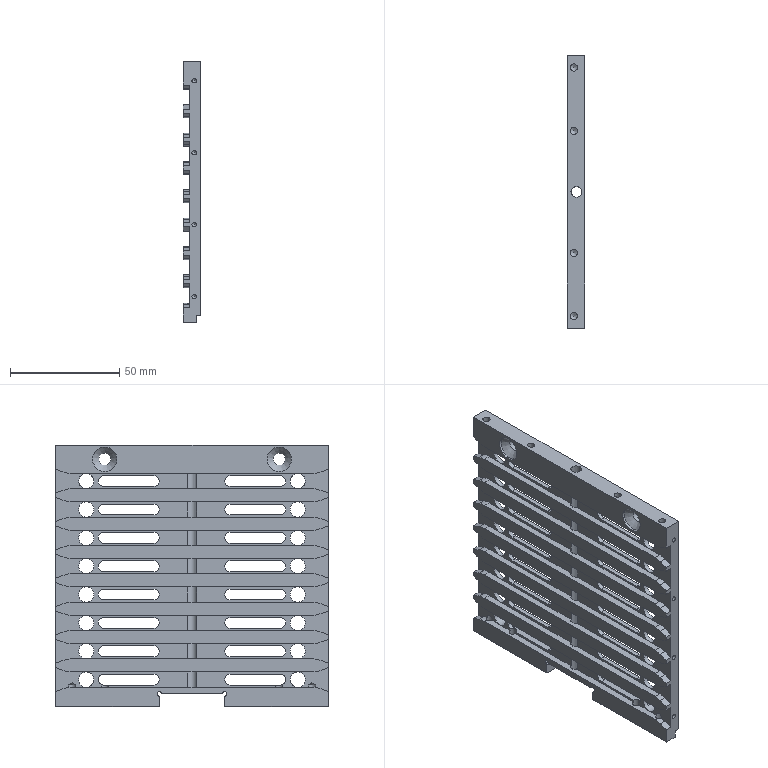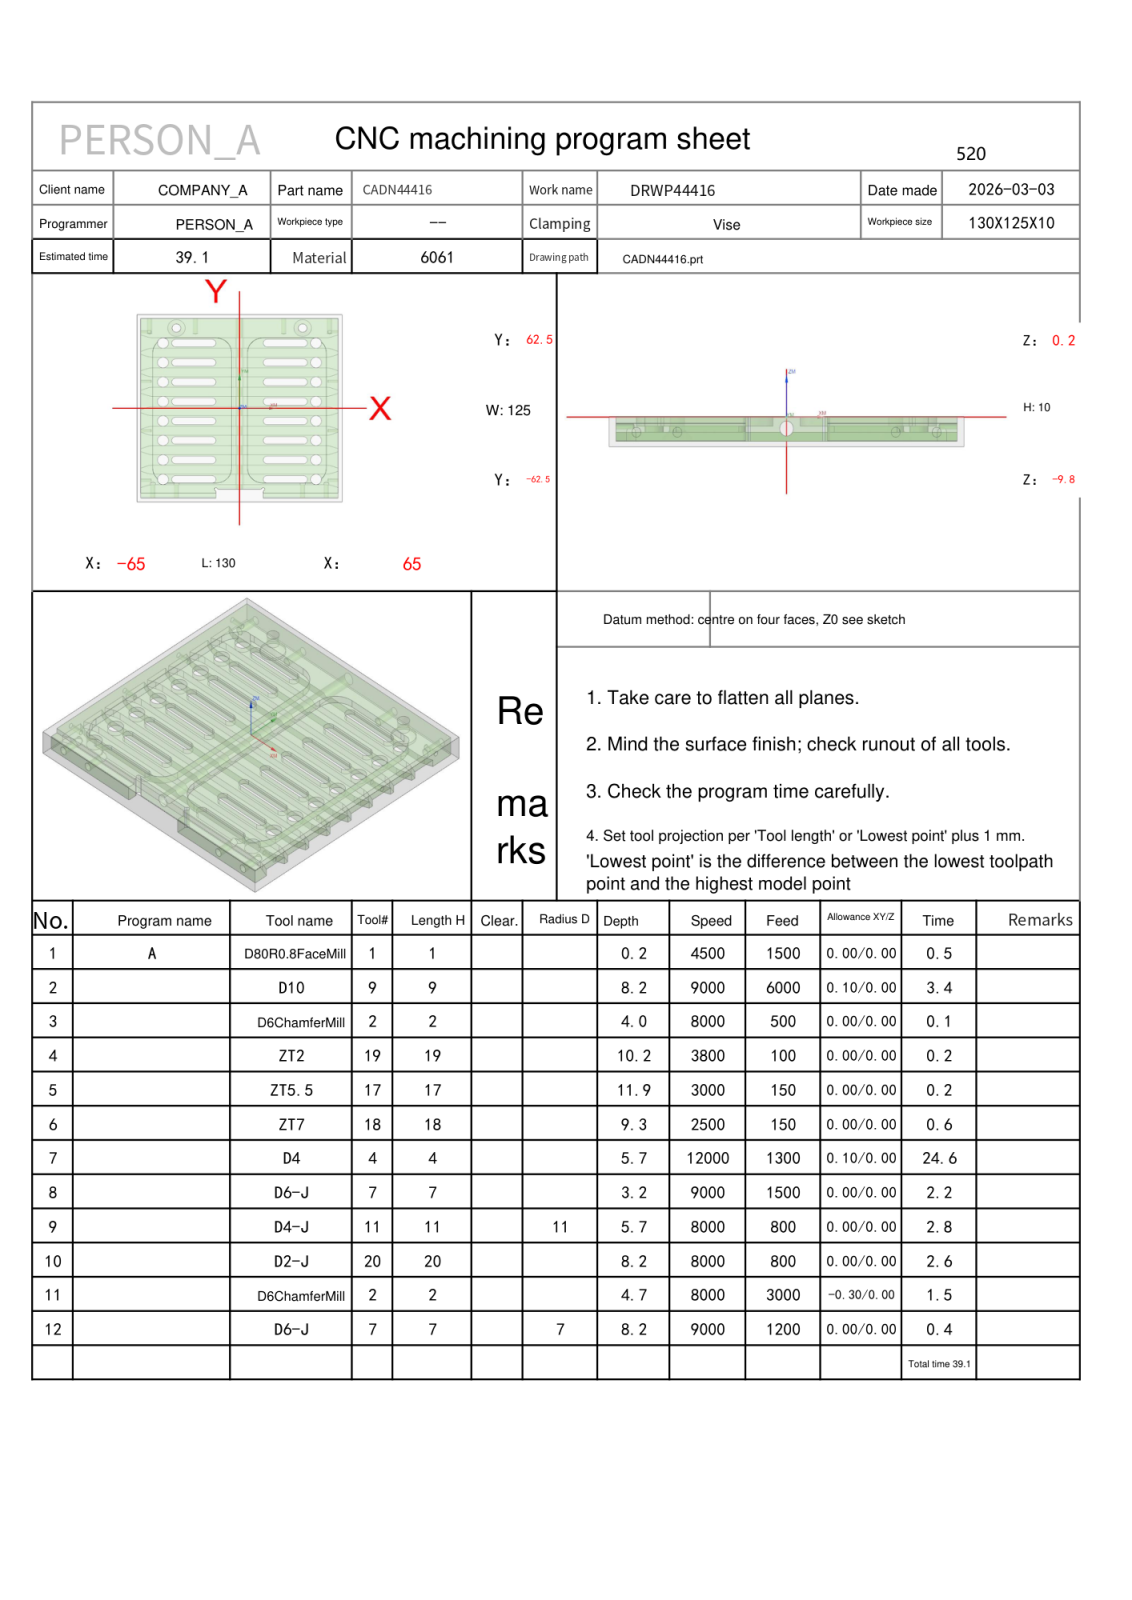NC program | NX | posted by the shop | part box 8 x 125 x 120 mm
Lines 4745 to 6257 of 11100:
N8 T07 M06
(D6-J  D=6. R=0. H=07 ce=0.30 di=0.00)
G00 G90 G54 X-8.3 Y-23.677 M03 S9000
G43 H07 Z30.
M08
Z-1.5
G01 Y-40. Z-2.07 F1500.
Y-40.366 Z-2.083
X-8.425 Y-41.338 Z-2.117
X-8.69 Y-42.281 Z-2.151
X-9.089 Y-43.176 Z-2.185
X-9.615 Y-44.003 Z-2.22
X-10.255 Y-44.745 Z-2.254
X-10.997 Y-45.385 Z-2.288
X-11.824 Y-45.911 Z-2.322
X-12.719 Y-46.31 Z-2.357
X-13.662 Y-46.575 Z-2.391
X-14.634 Y-46.7 Z-2.425
X-18.1 Z-2.546
Y-45.6 Z-2.584
X-30. Z-3.
X-39.9
Y-46.7
X-45.
G02 X-45.67 Y-46.666 I0.0 J6.7
G01 X-45.724 Y-46.661
G03 X-48.5 Y-44.6 I-2.776 J-.839
X-49.64 Y-44.833 I0.0 J-2.9
G01 X-49.679 Y-44.796
G02 X-51.7 Y-40. I4.679 J4.796
G01 Y37.
G02 X-50.238 Y41.178 I6.7 J0.0
G03 X-48.5 Y40.6 I1.738 J2.322
X-47.125 Y40.947 I0.0 J2.9
G01 X-46.815 Y41.114
X-46.711 Y41.217
G03 X-45.6 Y43.5 I-1.789 J2.283
G01 X-45.605 Y43.673
G02 X-45. Y43.7 I.605 J-6.673
G01 X-15.
G02 X-8.3 Y37. I0.0 J-6.7
G01 Y-40.
G02 X-15. Y-46.7 I-6.7 J0.0
G01 X-18.1
Y-45.6
X-30.
Y-41.4
X-39.9
G03 X-42.734 Y-42.5 I0.0 J-4.2
G01 X-43.459
G03 X-47.454 Y-40.477 I-5.041 J-5.
G02 X-47.5 Y-40. I2.454 J.477
G01 Y36.471
G03 X-45.134 Y37.249 I-1. J7.029
G01 X-44.281 Y37.708
X-43.881 Y38.108
G03 X-42.634 Y39.5 I-4.619 J5.392
G01 X-15.
G02 X-12.5 Y37. I0.0 J-2.5
G01 Y-40.
G02 X-15. Y-42.5 I-2.5 J0.0
G01 X-15.266
G03 X-18.1 Y-41.4 I-2.834 J-3.1
G01 X-30.
Y-37.2
X-39.901
G03 X-42.828 Y-37.727 I.001 J-8.4
X-43.3 Y-37.468 I-5.672 J-9.773
G01 Y33.468
X-43.143 Y33.551
X-41.747 Y34.302
X-41.013 Y35.037
G03 X-40.725 Y35.3 I-7.487 J8.463
G01 X-16.7
Y-37.317
G03 X-18.1 Y-37.2 I-1.4 J-8.283
G01 X-30.
Y-33.
X-39.1
Y31.01
X-39.01 Y31.1
X-20.9
Y-33.
X-30.
Y-28.8
X-34.9
Y26.9
X-25.1
Y-28.8
X-30.
Y-24.6
X-30.7
Y22.7
X-29.3
Y-24.6
X-30.
X-30.5
Y-28.2
Z-2.5
G00 Z30.
X51.7 Y-24.162
Z-1.5
G01 Y-40. Z-2.053
Y-40.366 Z-2.066
X51.647 Y-40.92 Z-2.085
X51.507 Y-41.639 Z-2.111
X51.254 Y-42.432 Z-2.14
X50.905 Y-43.187 Z-2.169
X50.465 Y-43.894 Z-2.198
X49.941 Y-44.54 Z-2.227
X49.64 Y-44.833 Z-2.242
X49.418 Y-44.739 Z-2.25
X48.872 Y-44.614 Z-2.27
X48.311 Y-44.596 Z-2.289
X47.834 Y-44.667 Z-2.306
X47.492 Y-44.77 Z-2.319
X47.055 Y-44.974 Z-2.336
X46.611 Y-45.287 Z-2.354
X46.271 Y-45.629 Z-2.371
X46. Y-46.01 Z-2.388
X45.794 Y-46.43 Z-2.404
X45.724 Y-46.661 Z-2.412
X45.336 Y-46.7 Z-2.426
X39.9 Z-2.616
Y-45.6 Z-2.654
X30. Z-3.
X18.1
Y-46.7
X15.
G02 X8.3 Y-40. I0.0 J6.7
G01 Y37.
G02 X15. Y43.7 I6.7 J0.0
G01 X45.
G02 X45.605 Y43.673 I0.0 J-6.7
G01 X45.6 Y43.5
G03 X46.711 Y41.217 I2.9 J0.0
G01 X46.815 Y41.114
X47.125 Y40.947
G03 X48.5 Y40.6 I1.375 J2.553
X50.238 Y41.178 I0.0 J2.9
G02 X51.7 Y37. I-5.238 J-4.178
G01 Y-40.
G02 X49.679 Y-44.796 I-6.7 J0.0
G01 X49.64 Y-44.833
G03 X48.5 Y-44.6 I-1.14 J-2.667
X45.724 Y-46.661 I0.0 J-2.9
G01 X45.67 Y-46.666
G02 X45. Y-46.7 I-.67 J6.666
G01 X39.9
Y-45.6
X30.
Y-41.4
X18.1
G03 X15.266 Y-42.5 I0.0 J-4.2
G01 X15.
G02 X12.5 Y-40. I0.0 J2.5
G01 Y37.
G02 X15. Y39.5 I2.5 J0.0
G01 X42.634
G03 X43.881 Y38.108 I5.866 J4.
G01 X44.281 Y37.708
X45.202 Y37.212
G03 X47.5 Y36.471 I3.298 J6.288
G01 Y-40.
G02 X47.454 Y-40.477 I-2.5 J0.0
G03 X43.459 Y-42.5 I1.046 J-7.023
G01 X42.734
G03 X39.9 Y-41.4 I-2.834 J-3.1
G01 X30.
Y-37.2
X18.1
G03 X16.7 Y-37.317 I0.0 J-8.4
G01 Y35.3
X40.725
G03 X41.013 Y35.037 I7.775 J8.2
G01 X41.748 Y34.302
X43.252 Y33.493
X43.3 Y33.468
Y-37.468
G03 X42.828 Y-37.727 I5.2 J-10.032
X39.9 Y-37.2 I-2.928 J-7.873
G01 X30.
Y-33.
X20.9
Y31.1
X39.01
X39.1 Y31.01
Y-33.
X30.
Y-28.8
X25.1
Y26.9
X34.9
Y-28.8
X30.
Y-24.6
X29.3
Y22.7
X30.7
Y-24.6
X30.
X29.5
Y-28.2
Z-2.5
G00 Z30.
G00 G90 X-48.132 Y42.816 M03 S9000
Z30.
Z-2.495
G01 Z-2.995 F1000.
G41 D07
X-48.466 Y43.665
X-48.568 Y43.675
G03 X-49.057 Y43.277 I0.0 J-.5
G01 X-49.179 Y42.692
X-49.849 Y42.049
G03 X-52. Y37. I4.849 J-5.049
G01 Y-40.
G03 X-49.888 Y-45.01 I7. J0.0
G01 X-48.857 Y-46.017
X-48.965 Y-47.121
X-48.968 Y-47.17
G03 X-48.516 Y-47.668 I.5 J0.0
G01 G40 X-48.417 Y-47.677
X-48.689 Y-47.55
G41 D07
X-48.618 Y-47.62
G03 X-48.268 Y-47.763 I.35 J.357
X-47.911 Y-47.613 I0.0 J.5
G01 X-47.134 Y-46.821
X-45.7 Y-46.965
G03 X-45. Y-47. I.7 J6.965
G01 X-15.
G03 X-8. Y-40. I0.0 J7.
G01 Y37.
G03 X-15. Y44. I-7. J0.0
G01 X-45.
G03 X-46.546 Y43.827 I0.0 J-7.
G01 X-47.452 Y43.622
X-48.007 Y43.842
X-48.192 Y43.878
G03 X-48.656 Y43.562 I0.0 J-.5
G01 G40 X-48.132 Y42.816
Z-2.495
G00 Z30.
X48.132
Z-2.495
G01 Z-2.995
G41 D07
X48.656 Y43.562
G03 X48.192 Y43.878 I-.465 J-.184
G01 X48.007 Y43.842
X47.452 Y43.622
X46.546 Y43.827
G03 X45. Y44. I-1.546 J-6.827
G01 X15.
G03 X8. Y37. I0.0 J-7.
G01 Y-40.
G03 X15. Y-47. I7. J0.0
G01 X45.
G03 X45.7 Y-46.965 I0.0 J7.
G01 X47.134 Y-46.821
X47.911 Y-47.613
G03 X48.268 Y-47.763 I.357 J.35
X48.618 Y-47.62 I0.0 J.5
G01 G40 X48.689 Y-47.55
X48.417 Y-47.677
G41 D07
X48.516 Y-47.668
G03 X48.968 Y-47.17 I-.049 J.498
G01 X48.965 Y-47.121
X48.857 Y-46.017
X49.888 Y-45.01
G03 X52. Y-40. I-4.888 J5.01
G01 Y37.
G03 X49.849 Y42.049 I-7. J0.0
G01 X49.179 Y42.692
X49.057 Y43.277
G03 X48.568 Y43.675 I-.49 J-.102
G01 X48.466 Y43.665
G40 X48.132 Y42.816
Z-2.495
G00 Z30.
G00 G90 X66.2 Y-60.6 M03 S9000
Z30.
Z-1.5
G01 Z-2. F1200.
G41 D07
Y-60.5
G03 X65.2 Y-59.5 I-1. J0.0
G01 X12.3
G03 X11.3 Y-60.5 I0.0 J-1.
G01 G40 Y-60.6
Z-1.5
G00 Z30.
X-11.3
Z-1.5
G01 Z-2.
G41 D07
Y-60.5
G03 X-12.3 Y-59.5 I-1. J0.0
G01 X-65.2
G03 X-66.2 Y-60.5 I0.0 J-1.
G01 G40 Y-60.6
Z-1.5
G00 Z30.
G91 G28 Z0.0
M05
M09
G91 G28 Z0.0
M01
N9 T11 M06
(D4-J  D=4. R=0. H=11 ce=0.00 di=0.00)
G00 G90 G54 X28.8 Y-34.75 M03 S8000
G43 H11 Z30.
M08
Z-5.
G01 Z-5.5 F500.
G41 D11
Y-34.8
G03 X29. Y-35. I.2 J0.0
G01 X40.5
G03 X41. Y-34.5 I0.0 J.5
X40.5 Y-34. I-.5 J0.0
G01 X17.5
G03 X17. Y-34.5 I0.0 J-.5
X17.5 Y-35. I.5 J0.0
G01 X29.
X29.5
G03 X29.7 Y-34.8 I0.0 J.2
G01 G40 Y-34.75
Z-5.
G00 Z30.
X28.8 Y-21.75
Z-5.
G01 Z-5.5
G41 D11
Y-21.8
G03 X29. Y-22. I.2 J0.0
G01 X40.5
G03 X41. Y-21.5 I0.0 J.5
X40.5 Y-21. I-.5 J0.0
G01 X17.5
G03 X17. Y-21.5 I0.0 J-.5
X17.5 Y-22. I.5 J0.0
G01 X29.
X29.5
G03 X29.7 Y-21.8 I0.0 J.2
G01 G40 Y-21.75
Z-5.
G00 Z30.
X29.2 Y-8.25
Z-5.
G01 Z-5.5
G41 D11
Y-8.2
G03 X29. Y-8. I-.2 J0.0
G01 X17.5
G03 X17. Y-8.5 I0.0 J-.5
X17.5 Y-9. I.5 J0.0
G01 X40.5
G03 X41. Y-8.5 I0.0 J.5
X40.5 Y-8. I-.5 J0.0
G01 X29.
X28.5
G03 X28.3 Y-8.2 I0.0 J-.2
G01 G40 Y-8.25
Z-5.
G00 Z30.
X29.2 Y4.75
Z-5.
G01 Z-5.5
G41 D11
Y4.8
G03 X29. Y5. I-.2 J0.0
G01 X17.5
G03 X17. Y4.5 I0.0 J-.5
X17.5 Y4. I.5 J0.0
G01 X40.5
G03 X41. Y4.5 I0.0 J.5
X40.5 Y5. I-.5 J0.0
G01 X29.
X28.5
G03 X28.3 Y4.8 I0.0 J-.2
G01 G40 Y4.75
Z-5.
G00 Z30.
X29.2 Y17.75
Z-5.
G01 Z-5.5
G41 D11
Y17.8
G03 X29. Y18. I-.2 J0.0
G01 X17.5
G03 X17. Y17.5 I0.0 J-.5
X17.5 Y17. I.5 J0.0
G01 X40.5
G03 X41. Y17.5 I0.0 J.5
X40.5 Y18. I-.5 J0.0
G01 X29.
X28.5
G03 X28.3 Y17.8 I0.0 J-.2
G01 G40 Y17.75
Z-5.
G00 Z30.
X29.2 Y30.75
Z-5.
G01 Z-5.5
G41 D11
Y30.8
G03 X29. Y31. I-.2 J0.0
G01 X17.5
G03 X17. Y30.5 I0.0 J-.5
X17.5 Y30. I.5 J0.0
G01 X40.5
G03 X41. Y30.5 I0.0 J.5
X40.5 Y31. I-.5 J0.0
G01 X29.
X28.5
G03 X28.3 Y30.8 I0.0 J-.2
G01 G40 Y30.75
Z-5.
G00 Z30.
X29.2 Y43.75
Z-5.
G01 Z-5.5
G41 D11
Y43.8
G03 X29. Y44. I-.2 J0.0
G01 X17.5
G03 X17. Y43.5 I0.0 J-.5
X17.5 Y43. I.5 J0.0
G01 X40.5
G03 X41. Y43.5 I0.0 J.5
X40.5 Y44. I-.5 J0.0
G01 X29.
X28.5
G03 X28.3 Y43.8 I0.0 J-.2
G01 G40 Y43.75
Z-5.
G00 Z30.
X-29.2 Y-34.75
Z-5.
G01 Z-5.5
G41 D11
Y-34.8
G03 X-29. Y-35. I.2 J0.0
G01 X-17.5
G03 X-17. Y-34.5 I0.0 J.5
X-17.5 Y-34. I-.5 J0.0
G01 X-40.5
G03 X-41. Y-34.5 I0.0 J-.5
X-40.5 Y-35. I.5 J0.0
G01 X-29.
X-28.5
G03 X-28.3 Y-34.8 I0.0 J.2
G01 G40 Y-34.75
Z-5.
G00 Z30.
X-28.8 Y-21.25
Z-5.
G01 Z-5.5
G41 D11
Y-21.2
G03 X-29. Y-21. I-.2 J0.0
G01 X-40.5
G03 X-41. Y-21.5 I0.0 J-.5
X-40.5 Y-22. I.5 J0.0
G01 X-17.5
G03 X-17. Y-21.5 I0.0 J.5
X-17.5 Y-21. I-.5 J0.0
G01 X-29.
X-29.5
G03 X-29.7 Y-21.2 I0.0 J-.2
G01 G40 Y-21.25
Z-5.
G00 Z30.
X-28.8 Y-8.25
Z-5.
G01 Z-5.5
G41 D11
Y-8.2
G03 X-29. Y-8. I-.2 J0.0
G01 X-40.5
G03 X-41. Y-8.5 I0.0 J-.5
X-40.5 Y-9. I.5 J0.0
G01 X-17.5
G03 X-17. Y-8.5 I0.0 J.5
X-17.5 Y-8. I-.5 J0.0
G01 X-29.
X-29.5
G03 X-29.7 Y-8.2 I0.0 J-.2
G01 G40 Y-8.25
Z-5.
G00 Z30.
X-28.8 Y4.75
Z-5.
G01 Z-5.5
G41 D11
Y4.8
G03 X-29. Y5. I-.2 J0.0
G01 X-40.5
G03 X-41. Y4.5 I0.0 J-.5
X-40.5 Y4. I.5 J0.0
G01 X-17.5
G03 X-17. Y4.5 I0.0 J.5
X-17.5 Y5. I-.5 J0.0
G01 X-29.
X-29.5
G03 X-29.7 Y4.8 I0.0 J-.2
G01 G40 Y4.75
Z-5.
G00 Z30.
X-29.2 Y17.25
Z-5.
G01 Z-5.5
G41 D11
Y17.2
G03 X-29. Y17. I.2 J0.0
G01 X-17.5
G03 X-17. Y17.5 I0.0 J.5
X-17.5 Y18. I-.5 J0.0
G01 X-40.5
G03 X-41. Y17.5 I0.0 J-.5
X-40.5 Y17. I.5 J0.0
G01 X-29.
X-28.5
G03 X-28.3 Y17.2 I0.0 J.2
G01 G40 Y17.25
Z-5.
G00 Z30.
X-28.8 Y30.75
Z-5.
G01 Z-5.5
G41 D11
Y30.8
G03 X-29. Y31. I-.2 J0.0
G01 X-40.5
G03 X-41. Y30.5 I0.0 J-.5
X-40.5 Y30. I.5 J0.0
G01 X-17.5
G03 X-17. Y30.5 I0.0 J.5
X-17.5 Y31. I-.5 J0.0
G01 X-29.
X-29.5
G03 X-29.7 Y30.8 I0.0 J-.2
G01 G40 Y30.75
Z-5.
G00 Z30.
X-28.8 Y43.75
Z-5.
G01 Z-5.5
G41 D11
Y43.8
G03 X-29. Y44. I-.2 J0.0
G01 X-40.5
G03 X-41. Y43.5 I0.0 J-.5
X-40.5 Y43. I.5 J0.0
G01 X-17.5
G03 X-17. Y43.5 I0.0 J.5
X-17.5 Y44. I-.5 J0.0
G01 X-29.
X-29.5
G03 X-29.7 Y43.8 I0.0 J-.2
G01 G40 Y43.75
Z-5.
G00 Z30.
G00 G90 X-29.2 Y-47.75 M03 S8000
Z30.
Z-2.25
G01 Z-2.75 F500.
G41 D11
Y-47.8
G03 X-29. Y-48. I.2 J0.0
G01 X-17.5
G03 X-17. Y-47.5 I0.0 J.5
X-17.5 Y-47. I-.5 J0.0
G01 X-40.5
G03 X-41. Y-47.5 I0.0 J-.5
X-40.5 Y-48. I.5 J0.0
G01 X-29.
X-28.5
G03 X-28.3 Y-47.8 I0.0 J.2
G01 G40 Y-47.75
Z-2.25
G00 Z.5
X-29.2
Z-5.
G01 Z-5.5
G41 D11
Y-47.8
G03 X-29. Y-48. I.2 J0.0
G01 X-17.5
G03 X-17. Y-47.5 I0.0 J.5
X-17.5 Y-47. I-.5 J0.0
G01 X-40.5
G03 X-41. Y-47.5 I0.0 J-.5
X-40.5 Y-48. I.5 J0.0
G01 X-29.
X-28.5
G03 X-28.3 Y-47.8 I0.0 J.2
G01 G40 Y-47.75
Z-5.
G00 Z30.
X28.8
Z-2.25
G01 Z-2.75
G41 D11
Y-47.8
G03 X29. Y-48. I.2 J0.0
G01 X40.5
G03 X41. Y-47.5 I0.0 J.5
X40.5 Y-47. I-.5 J0.0
G01 X17.5
G03 X17. Y-47.5 I0.0 J-.5
X17.5 Y-48. I.5 J0.0
G01 X29.
X29.5
G03 X29.7 Y-47.8 I0.0 J.2
G01 G40 Y-47.75
Z-2.25
G00 Z.5
X28.8
Z-5.
G01 Z-5.5
G41 D11
Y-47.8
G03 X29. Y-48. I.2 J0.0
G01 X40.5
G03 X41. Y-47.5 I0.0 J.5
X40.5 Y-47. I-.5 J0.0
G01 X17.5
G03 X17. Y-47.5 I0.0 J-.5
X17.5 Y-48. I.5 J0.0
G01 X29.
X29.5
G03 X29.7 Y-47.8 I0.0 J.2
G01 G40 Y-47.75
Z-5.
G00 Z30.
G00 G90 X-49.918 Y30.85 M03 S8000
Z30.
Z-2.5
G01 X-49.962 Y30.656 Z-2.51 F800.
X-49.965 Y30.379 Z-2.525
X-49.911 Y30.089 Z-2.54
X-49.801 Y29.816 Z-2.556
X-49.638 Y29.57 Z-2.571
X-49.43 Y29.362 Z-2.587
X-49.184 Y29.199 Z-2.602
X-48.911 Y29.089 Z-2.618
X-48.621 Y29.035 Z-2.633
X-48.379 Z-2.646
X-48.089 Y29.089 Z-2.661
X-47.816 Y29.199 Z-2.677
X-47.57 Y29.362 Z-2.692
X-47.362 Y29.57 Z-2.708
X-47.199 Y29.816 Z-2.723
X-47.089 Y30.089 Z-2.738
X-47.035 Y30.379 Z-2.754
Y30.621 Z-2.767
X-47.089 Y30.911 Z-2.782
X-47.199 Y31.184 Z-2.798
X-47.362 Y31.43 Z-2.813
X-47.57 Y31.638 Z-2.828
X-47.816 Y31.801 Z-2.844
X-48.089 Y31.911 Z-2.859
X-48.379 Y31.965 Z-2.875
X-48.621 Z-2.887
X-48.952 Y31.899 Z-2.905
X-49.26 Y31.759 Z-2.923
X-49.527 Y31.552 Z-2.941
X-49.74 Y31.29 Z-2.958
X-49.887 Y30.986 Z-2.976
X-49.962 Y30.656 Z-2.994
X-49.965 Y30.535 Z-3.
G41 D11
X-50. Y30.5
G03 X-48.5 Y29. Z-3.475 I1.5 J0.0
X-47. Y30.5 Z-3.95 I0.0 J1.5
X-48.5 Y32. Z-4.425 I-1.5 J0.0
X-50. Y30.5 Z-4.9 I0.0 J-1.5
X-48.5 Y29. I1.5 J0.0
X-47. Y30.5 I0.0 J1.5
X-48.5 Y32. I-1.5 J0.0
X-50. Y30.5 I0.0 J-1.5
X-49.947 Y30.105 I1.5 J0.0
G01 X-49.937 Y30.079
X-49.913 Y30.065
X-49.886 Y30.07
G40 X-49.837 Y30.083
Z-3.9
G00 Z30.
X-49.918 Y17.85
Z-2.5
G01 X-49.962 Y17.656 Z-2.51
X-49.965 Y17.379 Z-2.525
X-49.911 Y17.089 Z-2.54
X-49.801 Y16.816 Z-2.556
X-49.638 Y16.57 Z-2.571
X-49.43 Y16.362 Z-2.587
X-49.184 Y16.199 Z-2.602
X-48.911 Y16.089 Z-2.618
X-48.621 Y16.035 Z-2.633
X-48.379 Z-2.646
X-48.089 Y16.089 Z-2.661
X-47.816 Y16.199 Z-2.677
X-47.57 Y16.362 Z-2.692
X-47.362 Y16.57 Z-2.708
X-47.199 Y16.816 Z-2.723
X-47.089 Y17.089 Z-2.738
X-47.035 Y17.379 Z-2.754
Y17.621 Z-2.767
X-47.089 Y17.911 Z-2.782
X-47.199 Y18.184 Z-2.798
X-47.362 Y18.43 Z-2.813
X-47.57 Y18.638 Z-2.828
X-47.816 Y18.801 Z-2.844
X-48.089 Y18.911 Z-2.859
X-48.379 Y18.965 Z-2.875
X-48.621 Z-2.887
X-48.952 Y18.899 Z-2.905
X-49.26 Y18.759 Z-2.923
X-49.527 Y18.552 Z-2.941
X-49.74 Y18.29 Z-2.958
X-49.887 Y17.986 Z-2.976
X-49.962 Y17.656 Z-2.994
X-49.965 Y17.535 Z-3.
G41 D11
X-50. Y17.5
G03 X-48.5 Y16. Z-3.475 I1.5 J0.0
X-47. Y17.5 Z-3.95 I0.0 J1.5
X-48.5 Y19. Z-4.425 I-1.5 J0.0
X-50. Y17.5 Z-4.9 I0.0 J-1.5
X-48.5 Y16. I1.5 J0.0
X-47. Y17.5 I0.0 J1.5
X-48.5 Y19. I-1.5 J0.0
X-50. Y17.5 I0.0 J-1.5
X-49.947 Y17.105 I1.5 J0.0
G01 X-49.937 Y17.079
X-49.913 Y17.065
X-49.886 Y17.07
G40 X-49.837 Y17.083
Z-3.9
G00 Z30.
X-49.918 Y4.85
Z-2.5
G01 X-49.962 Y4.656 Z-2.51
X-49.965 Y4.379 Z-2.525
X-49.911 Y4.089 Z-2.54
X-49.801 Y3.816 Z-2.556
X-49.638 Y3.57 Z-2.571
X-49.43 Y3.362 Z-2.587
X-49.184 Y3.199 Z-2.602
X-48.911 Y3.089 Z-2.618
X-48.621 Y3.035 Z-2.633
X-48.379 Z-2.646
X-48.089 Y3.089 Z-2.661
X-47.816 Y3.199 Z-2.677
X-47.57 Y3.362 Z-2.692
X-47.362 Y3.57 Z-2.708
X-47.199 Y3.816 Z-2.723
X-47.089 Y4.089 Z-2.738
X-47.035 Y4.379 Z-2.754
Y4.621 Z-2.767
X-47.089 Y4.911 Z-2.782
X-47.199 Y5.184 Z-2.798
X-47.362 Y5.43 Z-2.813
X-47.57 Y5.638 Z-2.828
X-47.816 Y5.801 Z-2.844
X-48.089 Y5.911 Z-2.859
X-48.379 Y5.965 Z-2.875
X-48.621 Z-2.887
X-48.952 Y5.899 Z-2.905
X-49.26 Y5.759 Z-2.923
X-49.527 Y5.552 Z-2.941
X-49.74 Y5.29 Z-2.958
X-49.887 Y4.986 Z-2.976
X-49.962 Y4.656 Z-2.994
X-49.965 Y4.535 Z-3.
G41 D11
X-50. Y4.5
G03 X-48.5 Y3. Z-3.475 I1.5 J0.0
X-47. Y4.5 Z-3.95 I0.0 J1.5
X-48.5 Y6. Z-4.425 I-1.5 J0.0
X-50. Y4.5 Z-4.9 I0.0 J-1.5
X-48.5 Y3. I1.5 J0.0
X-47. Y4.5 I0.0 J1.5
X-48.5 Y6. I-1.5 J0.0
X-50. Y4.5 I0.0 J-1.5
X-49.947 Y4.105 I1.5 J0.0
G01 X-49.937 Y4.079
X-49.913 Y4.065
X-49.886 Y4.07
G40 X-49.837 Y4.083
Z-3.9
G00 Z30.
X-49.925 Y-8.15
Z-2.5
G01 X-49.962 Y-8.344 Z-2.51
X-49.965 Y-8.621 Z-2.525
X-49.911 Y-8.911 Z-2.54
X-49.801 Y-9.184 Z-2.556
X-49.638 Y-9.43 Z-2.571
X-49.43 Y-9.638 Z-2.587
X-49.184 Y-9.801 Z-2.602
X-48.911 Y-9.911 Z-2.618
X-48.621 Y-9.965 Z-2.633
X-48.379 Z-2.646
X-48.089 Y-9.911 Z-2.661
X-47.816 Y-9.801 Z-2.677
X-47.57 Y-9.638 Z-2.692
X-47.362 Y-9.43 Z-2.707
X-47.199 Y-9.184 Z-2.723
X-47.089 Y-8.911 Z-2.738
X-47.035 Y-8.621 Z-2.754
Y-8.379 Z-2.767
X-47.089 Y-8.089 Z-2.782
X-47.199 Y-7.816 Z-2.797
X-47.362 Y-7.57 Z-2.813
X-47.57 Y-7.362 Z-2.828
X-47.816 Y-7.199 Z-2.844
X-48.089 Y-7.089 Z-2.859
X-48.379 Y-7.035 Z-2.875
X-48.621 Z-2.887
X-48.89 Y-7.083 Z-2.902
X-49.145 Y-7.179 Z-2.916
X-49.378 Y-7.321 Z-2.93
X-49.581 Y-7.503 Z-2.945
X-49.73 Y-7.695 Z-2.957
X-49.841 Y-7.898 Z-2.969
X-49.919 Y-8.116 Z-2.982
X-49.962 Y-8.344 Z-2.994
X-49.965 Y-8.465 Z-3.
G41 D11
X-50. Y-8.5
G03 X-48.5 Y-10. Z-3.475 I1.5 J0.0
X-47. Y-8.5 Z-3.95 I0.0 J1.5
X-48.5 Y-7. Z-4.425 I-1.5 J0.0
X-49.683 Y-7.578 Z-4.7 I0.0 J-1.5
X-50. Y-8.5 Z-4.9 I1.183 J-.922
X-48.5 Y-10. I1.5 J0.0
X-47. Y-8.5 I0.0 J1.5
X-48.5 Y-7. I-1.5 J0.0
X-50. Y-8.5 I0.0 J-1.5
X-49.947 Y-8.895 I1.5 J0.0
G01 X-49.937 Y-8.921
X-49.913 Y-8.935
X-49.886 Y-8.93
G40 X-49.837 Y-8.917
Z-3.9
G00 Z30.
X-49.918 Y-21.15
Z-2.5
G01 X-49.962 Y-21.344 Z-2.51
X-49.965 Y-21.621 Z-2.525
X-49.911 Y-21.911 Z-2.54
X-49.801 Y-22.184 Z-2.556
X-49.638 Y-22.43 Z-2.571
X-49.43 Y-22.638 Z-2.587
X-49.184 Y-22.801 Z-2.602
X-48.911 Y-22.911 Z-2.618
X-48.621 Y-22.965 Z-2.633
X-48.379 Z-2.646
X-48.089 Y-22.911 Z-2.661
X-47.816 Y-22.801 Z-2.677
X-47.57 Y-22.638 Z-2.692
X-47.362 Y-22.43 Z-2.708
X-47.199 Y-22.184 Z-2.723
X-47.089 Y-21.911 Z-2.738
X-47.035 Y-21.621 Z-2.754
Y-21.379 Z-2.767
X-47.089 Y-21.089 Z-2.782
X-47.199 Y-20.816 Z-2.798
X-47.362 Y-20.57 Z-2.813
X-47.57 Y-20.362 Z-2.828
X-47.816 Y-20.199 Z-2.844
X-48.089 Y-20.089 Z-2.859
X-48.379 Y-20.035 Z-2.875
X-48.621 Z-2.887
X-48.952 Y-20.101 Z-2.905
X-49.26 Y-20.241 Z-2.923
X-49.527 Y-20.448 Z-2.941
X-49.74 Y-20.71 Z-2.958
X-49.887 Y-21.014 Z-2.976
X-49.962 Y-21.344 Z-2.994
X-49.965 Y-21.465 Z-3.
G41 D11
X-50. Y-21.5
G03 X-48.5 Y-23. Z-3.475 I1.5 J0.0
X-47. Y-21.5 Z-3.95 I0.0 J1.5
X-48.5 Y-20. Z-4.425 I-1.5 J0.0
X-50. Y-21.5 Z-4.9 I0.0 J-1.5
X-48.5 Y-23. I1.5 J0.0
X-47. Y-21.5 I0.0 J1.5
X-48.5 Y-20. I-1.5 J0.0
X-50. Y-21.5 I0.0 J-1.5
X-49.947 Y-21.895 I1.5 J0.0
G01 X-49.937 Y-21.921
X-49.913 Y-21.935
X-49.886 Y-21.93
G40 X-49.837 Y-21.917
Z-3.9
G00 Z30.
X-49.918 Y-34.15
Z-2.5
G01 X-49.962 Y-34.344 Z-2.51
X-49.965 Y-34.621 Z-2.525
X-49.911 Y-34.911 Z-2.54
X-49.801 Y-35.184 Z-2.556
X-49.638 Y-35.43 Z-2.571
X-49.43 Y-35.638 Z-2.587
X-49.184 Y-35.801 Z-2.602
X-48.911 Y-35.911 Z-2.618
X-48.621 Y-35.965 Z-2.633
X-48.379 Z-2.646
X-48.089 Y-35.911 Z-2.661
X-47.816 Y-35.801 Z-2.677
X-47.57 Y-35.638 Z-2.692
X-47.362 Y-35.43 Z-2.708
X-47.199 Y-35.184 Z-2.723
X-47.089 Y-34.911 Z-2.738
X-47.035 Y-34.621 Z-2.754
Y-34.379 Z-2.767
X-47.089 Y-34.089 Z-2.782
X-47.199 Y-33.816 Z-2.798
X-47.362 Y-33.57 Z-2.813
X-47.57 Y-33.362 Z-2.828
X-47.816 Y-33.199 Z-2.844
X-48.089 Y-33.089 Z-2.859
X-48.379 Y-33.035 Z-2.875
X-48.621 Z-2.887
X-48.952 Y-33.101 Z-2.905
X-49.26 Y-33.241 Z-2.923
X-49.527 Y-33.448 Z-2.941
X-49.74 Y-33.71 Z-2.958
X-49.887 Y-34.014 Z-2.976
X-49.962 Y-34.344 Z-2.994
X-49.965 Y-34.465 Z-3.
G41 D11
X-50. Y-34.5
G03 X-48.5 Y-36. Z-3.475 I1.5 J0.0
X-47. Y-34.5 Z-3.95 I0.0 J1.5
X-48.5 Y-33. Z-4.425 I-1.5 J0.0
X-50. Y-34.5 Z-4.9 I0.0 J-1.5
X-48.5 Y-36. I1.5 J0.0
X-47. Y-34.5 I0.0 J1.5
X-48.5 Y-33. I-1.5 J0.0
X-50. Y-34.5 I0.0 J-1.5
X-49.947 Y-34.895 I1.5 J0.0
G01 X-49.937 Y-34.921
X-49.913 Y-34.935
X-49.886 Y-34.93
G40 X-49.837 Y-34.917
Z-3.9
G00 Z30.
X49.918 Y-34.85
Z-2.5
G01 X49.962 Y-34.656 Z-2.51
X49.965 Y-34.379 Z-2.525
X49.911 Y-34.089 Z-2.54
X49.801 Y-33.816 Z-2.556
X49.638 Y-33.57 Z-2.571
X49.43 Y-33.362 Z-2.587
X49.184 Y-33.199 Z-2.602
X48.911 Y-33.089 Z-2.618
X48.621 Y-33.035 Z-2.633
X48.379 Z-2.646
X48.089 Y-33.089 Z-2.661
X47.816 Y-33.199 Z-2.677
X47.57 Y-33.362 Z-2.692
X47.362 Y-33.57 Z-2.708
X47.199 Y-33.816 Z-2.723
X47.089 Y-34.089 Z-2.738
X47.035 Y-34.379 Z-2.754
Y-34.621 Z-2.767
X47.089 Y-34.911 Z-2.782
X47.199 Y-35.184 Z-2.798
X47.362 Y-35.43 Z-2.813
X47.57 Y-35.638 Z-2.828
X47.816 Y-35.801 Z-2.844
X48.089 Y-35.911 Z-2.859
X48.379 Y-35.965 Z-2.875
X48.621 Z-2.887
X48.952 Y-35.899 Z-2.905
X49.26 Y-35.759 Z-2.923
X49.527 Y-35.552 Z-2.941
X49.74 Y-35.29 Z-2.958
X49.887 Y-34.986 Z-2.976
X49.962 Y-34.656 Z-2.994
X49.965 Y-34.535 Z-3.
G41 D11
X50. Y-34.5
G03 X48.5 Y-33. Z-3.475 I-1.5 J0.0
X47. Y-34.5 Z-3.95 I0.0 J-1.5
X48.5 Y-36. Z-4.425 I1.5 J0.0
X50. Y-34.5 Z-4.9 I0.0 J1.5
X48.5 Y-33. I-1.5 J0.0
X47. Y-34.5 I0.0 J-1.5
X48.5 Y-36. I1.5 J0.0
X50. Y-34.5 I0.0 J1.5
X49.947 Y-34.105 I-1.5 J0.0
G01 X49.937 Y-34.079
X49.913 Y-34.065
X49.886 Y-34.07
G40 X49.837 Y-34.083
Z-3.9
G00 Z30.
X49.918 Y-21.85
Z-2.5
G01 X49.962 Y-21.656 Z-2.51
X49.965 Y-21.379 Z-2.525
X49.911 Y-21.089 Z-2.54
X49.801 Y-20.816 Z-2.556
X49.638 Y-20.57 Z-2.571
X49.43 Y-20.362 Z-2.587
X49.184 Y-20.199 Z-2.602
X48.911 Y-20.089 Z-2.618
X48.621 Y-20.035 Z-2.633
X48.379 Z-2.646
X48.089 Y-20.089 Z-2.661
X47.816 Y-20.199 Z-2.677
X47.57 Y-20.362 Z-2.692
X47.362 Y-20.57 Z-2.708
X47.199 Y-20.816 Z-2.723
X47.089 Y-21.089 Z-2.738
X47.035 Y-21.379 Z-2.754
Y-21.621 Z-2.767
X47.089 Y-21.911 Z-2.782
X47.199 Y-22.184 Z-2.798
X47.362 Y-22.43 Z-2.813
X47.57 Y-22.638 Z-2.828
X47.816 Y-22.801 Z-2.844
X48.089 Y-22.911 Z-2.859
X48.379 Y-22.965 Z-2.875
X48.621 Z-2.887
X48.952 Y-22.899 Z-2.905
X49.26 Y-22.759 Z-2.923
X49.527 Y-22.552 Z-2.941
X49.74 Y-22.29 Z-2.958
X49.887 Y-21.986 Z-2.976
X49.962 Y-21.656 Z-2.994
X49.965 Y-21.535 Z-3.
G41 D11
X50. Y-21.5
G03 X48.5 Y-20. Z-3.475 I-1.5 J0.0
X47. Y-21.5 Z-3.95 I0.0 J-1.5
X48.5 Y-23. Z-4.425 I1.5 J0.0
X50. Y-21.5 Z-4.9 I0.0 J1.5
X48.5 Y-20. I-1.5 J0.0
X47. Y-21.5 I0.0 J-1.5
X48.5 Y-23. I1.5 J0.0
X50. Y-21.5 I0.0 J1.5
X49.947 Y-21.105 I-1.5 J0.0
G01 X49.937 Y-21.079
X49.913 Y-21.065
X49.886 Y-21.07
G40 X49.837 Y-21.083
Z-3.9
G00 Z30.
X49.918 Y-8.85
Z-2.5
G01 X49.962 Y-8.656 Z-2.51
X49.965 Y-8.379 Z-2.525
X49.911 Y-8.089 Z-2.54
X49.801 Y-7.816 Z-2.556
X49.638 Y-7.57 Z-2.571
X49.43 Y-7.362 Z-2.587
X49.184 Y-7.199 Z-2.602
X48.911 Y-7.089 Z-2.618
X48.621 Y-7.035 Z-2.633
X48.379 Z-2.646
X48.089 Y-7.089 Z-2.661
X47.816 Y-7.199 Z-2.677
X47.57 Y-7.362 Z-2.692
X47.362 Y-7.57 Z-2.708
X47.199 Y-7.816 Z-2.723
X47.089 Y-8.089 Z-2.738
X47.035 Y-8.379 Z-2.754
Y-8.621 Z-2.767
X47.089 Y-8.911 Z-2.782
X47.199 Y-9.184 Z-2.798
X47.362 Y-9.43 Z-2.813
X47.57 Y-9.638 Z-2.828
X47.816 Y-9.801 Z-2.844
X48.089 Y-9.911 Z-2.859
X48.379 Y-9.965 Z-2.875
X48.621 Z-2.887
X48.952 Y-9.899 Z-2.905
X49.26 Y-9.759 Z-2.923
X49.527 Y-9.552 Z-2.941
X49.74 Y-9.29 Z-2.958
X49.887 Y-8.986 Z-2.976
X49.962 Y-8.656 Z-2.994
X49.965 Y-8.535 Z-3.
G41 D11
X50. Y-8.5
G03 X48.5 Y-7. Z-3.475 I-1.5 J0.0
X47. Y-8.5 Z-3.95 I0.0 J-1.5
X48.5 Y-10. Z-4.425 I1.5 J0.0
X50. Y-8.5 Z-4.9 I0.0 J1.5
X48.5 Y-7. I-1.5 J0.0
X47. Y-8.5 I0.0 J-1.5
X48.5 Y-10. I1.5 J0.0
X50. Y-8.5 I0.0 J1.5
X49.947 Y-8.105 I-1.5 J0.0
G01 X49.937 Y-8.079
X49.913 Y-8.065
X49.886 Y-8.07
G40 X49.837 Y-8.083
Z-3.9
G00 Z30.
X49.918 Y4.15
Z-2.5
G01 X49.962 Y4.344 Z-2.51
X49.965 Y4.621 Z-2.525
X49.911 Y4.911 Z-2.54
X49.801 Y5.184 Z-2.556
X49.638 Y5.43 Z-2.571
X49.43 Y5.638 Z-2.587
X49.184 Y5.801 Z-2.602
X48.911 Y5.911 Z-2.618
X48.621 Y5.965 Z-2.633
X48.379 Z-2.646
X48.089 Y5.911 Z-2.661
X47.816 Y5.801 Z-2.677
X47.57 Y5.638 Z-2.692
X47.362 Y5.43 Z-2.708
X47.199 Y5.184 Z-2.723
X47.089 Y4.911 Z-2.738
X47.035 Y4.621 Z-2.754
Y4.379 Z-2.767
X47.089 Y4.089 Z-2.782
X47.199 Y3.816 Z-2.798
X47.362 Y3.57 Z-2.813
X47.57 Y3.362 Z-2.828
X47.816 Y3.199 Z-2.844
X48.089 Y3.089 Z-2.859
X48.379 Y3.035 Z-2.875
X48.621 Z-2.887
X48.952 Y3.101 Z-2.905
X49.26 Y3.241 Z-2.923
X49.527 Y3.448 Z-2.941
X49.74 Y3.71 Z-2.958
X49.887 Y4.014 Z-2.976
X49.962 Y4.344 Z-2.994
X49.965 Y4.465 Z-3.
G41 D11
X50. Y4.5
G03 X48.5 Y6. Z-3.475 I-1.5 J0.0
X47. Y4.5 Z-3.95 I0.0 J-1.5
X48.5 Y3. Z-4.425 I1.5 J0.0
X50. Y4.5 Z-4.9 I0.0 J1.5
X48.5 Y6. I-1.5 J0.0
X47. Y4.5 I0.0 J-1.5
X48.5 Y3. I1.5 J0.0
X50. Y4.5 I0.0 J1.5
X49.947 Y4.895 I-1.5 J0.0
G01 X49.937 Y4.921
X49.913 Y4.935
X49.886 Y4.93
G40 X49.837 Y4.917
Z-3.9
G00 Z30.
X49.918 Y17.15
Z-2.5
G01 X49.962 Y17.344 Z-2.51
X49.965 Y17.621 Z-2.525
X49.911 Y17.911 Z-2.54
X49.801 Y18.184 Z-2.556
X49.638 Y18.43 Z-2.571
X49.43 Y18.638 Z-2.587
X49.184 Y18.801 Z-2.602
X48.911 Y18.911 Z-2.618
X48.621 Y18.965 Z-2.633
X48.379 Z-2.646
X48.089 Y18.911 Z-2.661
X47.816 Y18.801 Z-2.677
X47.57 Y18.638 Z-2.692
X47.362 Y18.43 Z-2.708
X47.199 Y18.184 Z-2.723
X47.089 Y17.911 Z-2.738
X47.035 Y17.621 Z-2.754
Y17.379 Z-2.767
X47.089 Y17.089 Z-2.782
X47.199 Y16.816 Z-2.798
X47.362 Y16.57 Z-2.813
X47.57 Y16.362 Z-2.828
X47.816 Y16.199 Z-2.844
X48.089 Y16.089 Z-2.859
X48.379 Y16.035 Z-2.875
X48.621 Z-2.887
X48.952 Y16.101 Z-2.905
X49.26 Y16.241 Z-2.923
X49.527 Y16.448 Z-2.941
X49.74 Y16.71 Z-2.958
X49.887 Y17.014 Z-2.976
X49.962 Y17.344 Z-2.994
X49.965 Y17.465 Z-3.
G41 D11
X50. Y17.5
G03 X48.5 Y19. Z-3.475 I-1.5 J0.0
X47. Y17.5 Z-3.95 I0.0 J-1.5
X48.5 Y16. Z-4.425 I1.5 J0.0
X50. Y17.5 Z-4.9 I0.0 J1.5
X48.5 Y19. I-1.5 J0.0
X47. Y17.5 I0.0 J-1.5
X48.5 Y16. I1.5 J0.0
X50. Y17.5 I0.0 J1.5
X49.947 Y17.895 I-1.5 J0.0
G01 X49.937 Y17.921
X49.913 Y17.935
X49.886 Y17.93
G40 X49.837 Y17.917
Z-3.9
G00 Z30.
X49.918 Y30.15
Z-2.5
G01 X49.962 Y30.344 Z-2.51
X49.965 Y30.621 Z-2.525
X49.911 Y30.911 Z-2.54
X49.801 Y31.184 Z-2.556
X49.638 Y31.43 Z-2.571
X49.43 Y31.638 Z-2.587
X49.184 Y31.801 Z-2.602
X48.911 Y31.911 Z-2.618
X48.621 Y31.965 Z-2.633
X48.379 Z-2.646
X48.089 Y31.911 Z-2.661
X47.816 Y31.801 Z-2.677
X47.57 Y31.638 Z-2.692
X47.362 Y31.43 Z-2.708
X47.199 Y31.184 Z-2.723
X47.089 Y30.911 Z-2.738
X47.035 Y30.621 Z-2.754
Y30.379 Z-2.767
X47.089 Y30.089 Z-2.782
X47.199 Y29.816 Z-2.798
X47.362 Y29.57 Z-2.813
X47.57 Y29.362 Z-2.828
X47.816 Y29.199 Z-2.844
X48.089 Y29.089 Z-2.859
X48.379 Y29.035 Z-2.875
X48.621 Z-2.887
X48.952 Y29.101 Z-2.905
X49.26 Y29.241 Z-2.923
X49.527 Y29.448 Z-2.941
X49.74 Y29.71 Z-2.958
X49.887 Y30.014 Z-2.976
X49.962 Y30.344 Z-2.994
X49.965 Y30.465 Z-3.
G41 D11
X50. Y30.5
G03 X48.5 Y32. Z-3.475 I-1.5 J0.0
X47. Y30.5 Z-3.95 I0.0 J-1.5
X48.5 Y29. Z-4.425 I1.5 J0.0
X50. Y30.5 Z-4.9 I0.0 J1.5
X48.5 Y32. I-1.5 J0.0
X47. Y30.5 I0.0 J-1.5
X48.5 Y29. I1.5 J0.0
X50. Y30.5 I0.0 J1.5
X49.947 Y30.895 I-1.5 J0.0
G01 X49.937 Y30.921
X49.913 Y30.935
X49.886 Y30.93
G40 X49.837 Y30.917
Z-3.9
G00 Z30.
G00 G90 X-48.85 Y-48.918 M03 S8000
Z30.
Z.5
G01 X-48.656 Y-48.962 Z.49 F800.
X-48.379 Y-48.965 Z.475
X-48.089 Y-48.911 Z.46
X-47.816 Y-48.801 Z.444
X-47.57 Y-48.638 Z.429
X-47.362 Y-48.43 Z.413
X-47.199 Y-48.184 Z.398
X-47.089 Y-47.911 Z.382
X-47.035 Y-47.621 Z.367
Y-47.379 Z.354
X-47.089 Y-47.089 Z.339
X-47.199 Y-46.816 Z.323
X-47.362 Y-46.57 Z.308
X-47.57 Y-46.362 Z.292
X-47.816 Y-46.199 Z.277
X-48.089 Y-46.089 Z.262
X-48.379 Y-46.035 Z.246
X-48.621 Z.233
X-48.911 Y-46.089 Z.218
X-49.184 Y-46.199 Z.202
X-49.43 Y-46.362 Z.187
X-49.638 Y-46.57 Z.172
X-49.801 Y-46.816 Z.156
X-49.911 Y-47.089 Z.141
X-49.965 Y-47.379 Z.125
Y-47.621 Z.113
X-49.899 Y-47.952 Z.095
X-49.759 Y-48.26 Z.077
X-49.552 Y-48.527 Z.059
X-49.29 Y-48.74 Z.042
X-48.986 Y-48.887 Z.024
X-48.656 Y-48.962 Z.006
X-48.535 Y-48.965 Z0.0
G41 D11
X-48.5 Y-49.
G03 X-47. Y-47.5 Z-.408 I0.0 J1.5
X-48.5 Y-46. Z-.817 I-1.5 J0.0
X-50. Y-47.5 Z-1.225 I0.0 J-1.5
X-48.5 Y-49. Z-1.633 I1.5 J0.0
X-47. Y-47.5 Z-2.042 I0.0 J1.5
X-48.5 Y-46. Z-2.45 I-1.5 J0.0
X-50. Y-47.5 Z-2.858 I0.0 J-1.5
X-48.5 Y-49. Z-3.267 I1.5 J0.0
X-47. Y-47.5 Z-3.675 I0.0 J1.5
X-48.5 Y-46. Z-4.083 I-1.5 J0.0
X-50. Y-47.5 Z-4.492 I0.0 J-1.5
X-48.5 Y-49. Z-4.9 I1.5 J0.0
X-47. Y-47.5 I0.0 J1.5
X-48.5 Y-46. I-1.5 J0.0
X-50. Y-47.5 I0.0 J-1.5
X-48.5 Y-49. I1.5 J0.0
X-48.105 Y-48.947 I0.0 J1.5
G01 X-48.079 Y-48.937
X-48.065 Y-48.913
X-48.07 Y-48.886
G40 X-48.083 Y-48.837
Z-3.9
G00 Z30.
X-49.918 Y43.85
Z.5
G01 X-49.962 Y43.656 Z.49
X-49.965 Y43.379 Z.475
X-49.911 Y43.089 Z.46
X-49.801 Y42.816 Z.444
X-49.638 Y42.57 Z.429
X-49.43 Y42.362 Z.413
X-49.184 Y42.199 Z.398
X-48.911 Y42.089 Z.382
X-48.621 Y42.035 Z.367
X-48.379 Z.354
X-48.089 Y42.089 Z.339
X-47.816 Y42.199 Z.323
X-47.57 Y42.362 Z.308
X-47.362 Y42.57 Z.292
X-47.199 Y42.816 Z.277
X-47.089 Y43.089 Z.262
X-47.035 Y43.379 Z.246
Y43.621 Z.233
X-47.089 Y43.911 Z.218
X-47.199 Y44.184 Z.202
X-47.362 Y44.43 Z.187
X-47.57 Y44.638 Z.172
X-47.816 Y44.801 Z.156
X-48.089 Y44.911 Z.141
X-48.379 Y44.965 Z.125
X-48.621 Z.113
X-48.952 Y44.899 Z.095
X-49.26 Y44.759 Z.077
X-49.527 Y44.552 Z.059
X-49.74 Y44.29 Z.042
X-49.887 Y43.986 Z.024
X-49.962 Y43.656 Z.006
X-49.965 Y43.535 Z0.0
G41 D11
X-50. Y43.5
G03 X-48.5 Y42. Z-.408 I1.5 J0.0
X-47. Y43.5 Z-.817 I0.0 J1.5
X-48.5 Y45. Z-1.225 I-1.5 J0.0
X-50. Y43.5 Z-1.633 I0.0 J-1.5
X-48.5 Y42. Z-2.042 I1.5 J0.0
X-47. Y43.5 Z-2.45 I0.0 J1.5
X-48.5 Y45. Z-2.858 I-1.5 J0.0
X-50. Y43.5 Z-3.267 I0.0 J-1.5
X-48.5 Y42. Z-3.675 I1.5 J0.0
X-47. Y43.5 Z-4.083 I0.0 J1.5
X-48.5 Y45. Z-4.492 I-1.5 J0.0
X-50. Y43.5 Z-4.9 I0.0 J-1.5
X-48.5 Y42. I1.5 J0.0
X-47. Y43.5 I0.0 J1.5
X-48.5 Y45. I-1.5 J0.0
X-50. Y43.5 I0.0 J-1.5
X-49.947 Y43.105 I1.5 J0.0
G01 X-49.937 Y43.079
X-49.913 Y43.065
X-49.886 Y43.07
G40 X-49.837 Y43.083
Z-3.9
G00 Z30.
X49.918 Y43.15
Z.5
G01 X49.962 Y43.344 Z.49
X49.965 Y43.621 Z.475
X49.911 Y43.911 Z.46
X49.801 Y44.184 Z.444
X49.638 Y44.43 Z.429
X49.43 Y44.638 Z.413
X49.184 Y44.801 Z.398
X48.911 Y44.911 Z.382
X48.621 Y44.965 Z.367
X48.379 Z.354
X48.089 Y44.911 Z.339
X47.816 Y44.801 Z.323
X47.57 Y44.638 Z.308
X47.362 Y44.43 Z.292
X47.199 Y44.184 Z.277
X47.089 Y43.911 Z.262
X47.035 Y43.621 Z.246
Y43.379 Z.233
X47.089 Y43.089 Z.218
X47.199 Y42.816 Z.202
X47.362 Y42.57 Z.187
X47.57 Y42.362 Z.172
X47.816 Y42.199 Z.156
X48.089 Y42.089 Z.141
X48.379 Y42.035 Z.125
X48.621 Z.113
X48.952 Y42.101 Z.095
X49.26 Y42.241 Z.077
X49.527 Y42.448 Z.059
X49.74 Y42.71 Z.042
X49.887 Y43.014 Z.024
X49.962 Y43.344 Z.006
X49.965 Y43.465 Z0.0
G41 D11
X50. Y43.5
G03 X48.5 Y45. Z-.408 I-1.5 J0.0
X47. Y43.5 Z-.817 I0.0 J-1.5
X48.5 Y42. Z-1.225 I1.5 J0.0
X50. Y43.5 Z-1.633 I0.0 J1.5
X48.5 Y45. Z-2.042 I-1.5 J0.0
X47. Y43.5 Z-2.45 I0.0 J-1.5
X48.5 Y42. Z-2.858 I1.5 J0.0
X50. Y43.5 Z-3.267 I0.0 J1.5
X48.5 Y45. Z-3.675 I-1.5 J0.0
X47. Y43.5 Z-4.083 I0.0 J-1.5
X48.5 Y42. Z-4.492 I1.5 J0.0
X50. Y43.5 Z-4.9 I0.0 J1.5
X48.5 Y45. I-1.5 J0.0
X47. Y43.5 I0.0 J-1.5
X48.5 Y42. I1.5 J0.0
X50. Y43.5 I0.0 J1.5
X49.947 Y43.895 I-1.5 J0.0
G01 X49.937 Y43.921
X49.913 Y43.935
X49.886 Y43.93
G40 X49.837 Y43.917
Z-3.9
G00 Z30.
X48.15 Y-48.918
Z.5
G01 X48.344 Y-48.962 Z.49
X48.621 Y-48.965 Z.475
X48.911 Y-48.911 Z.46
X49.184 Y-48.801 Z.444
X49.43 Y-48.638 Z.429
X49.638 Y-48.43 Z.413
X49.801 Y-48.184 Z.398
X49.911 Y-47.911 Z.382
X49.965 Y-47.621 Z.367
Y-47.379 Z.354
X49.911 Y-47.089 Z.339
X49.801 Y-46.816 Z.323
X49.638 Y-46.57 Z.308
X49.43 Y-46.362 Z.292
X49.184 Y-46.199 Z.277
X48.911 Y-46.089 Z.262
X48.621 Y-46.035 Z.246
X48.379 Z.233
X48.089 Y-46.089 Z.218
X47.816 Y-46.199 Z.202
X47.57 Y-46.362 Z.187
X47.362 Y-46.57 Z.172
X47.199 Y-46.816 Z.156
X47.089 Y-47.089 Z.141
X47.035 Y-47.379 Z.125
Y-47.621 Z.113
X47.101 Y-47.952 Z.095
X47.241 Y-48.26 Z.077
X47.448 Y-48.527 Z.059
X47.71 Y-48.74 Z.042
X48.014 Y-48.887 Z.024
X48.344 Y-48.962 Z.006
X48.465 Y-48.965 Z0.0
G41 D11
X48.5 Y-49.
G03 X50. Y-47.5 Z-.408 I0.0 J1.5
X48.5 Y-46. Z-.817 I-1.5 J0.0
X47. Y-47.5 Z-1.225 I0.0 J-1.5
X48.5 Y-49. Z-1.633 I1.5 J0.0
X50. Y-47.5 Z-2.042 I0.0 J1.5
X48.5 Y-46. Z-2.45 I-1.5 J0.0
X47. Y-47.5 Z-2.858 I0.0 J-1.5
X48.5 Y-49. Z-3.267 I1.5 J0.0
X50. Y-47.5 Z-3.675 I0.0 J1.5
X48.5 Y-46. Z-4.083 I-1.5 J0.0
X47. Y-47.5 Z-4.492 I0.0 J-1.5
X48.5 Y-49. Z-4.9 I1.5 J0.0
X50. Y-47.5 I0.0 J1.5
X48.5 Y-46. I-1.5 J0.0
X47. Y-47.5 I0.0 J-1.5
X48.5 Y-49. I1.5 J0.0
X48.895 Y-48.947 I0.0 J1.5
G01 X48.921 Y-48.937
X48.935 Y-48.913
X48.93 Y-48.886
G40 X48.917 Y-48.837
Z-3.9
G00 Z30.
G91 G28 Z0.0
M05
M09
G91 G28 Z0.0
M01